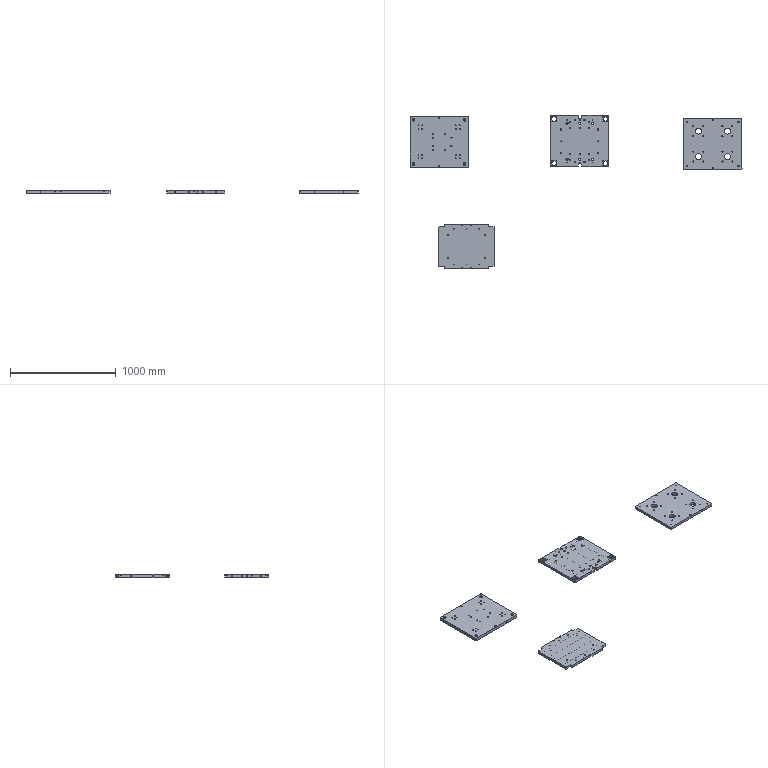NC program | Mastercam | posted with a generic post | part box 3140 x 1452 x 30 mm
Lines 6154 to 6493 of 6493:
N2080 T7 M6
N2090 G0 G90 G17 G54 X-248.05 Y-208.6 A0. S6000 M3
N2100 G43 H7 Z50. M8
N2110 Z1.2
N2120 G1 Z-1.25 F600.
N2130 X-248.45 F1000.
N2140 G3 X-248.85 Y-209. I0. J-.4
N2150 X-242. Y-215.85 I6.85 J0.
N2160 X-235.15 Y-209. I0. J6.85
N2170 X-242. Y-202.15 I-6.85 J0.
N2180 X-248.85 Y-209. I0. J-6.85
N2190 X-248.832 Y-209.5 I6.85 J0.
N2200 X-248.433 Y-209.87 I.399 J.03
N2210 X-248.404 Y-209.869 I0. J.4
N2220 G1 X-248.005 Y-209.84
N2230 G0 Z50.
N2240 X-245.55 Y-208.6
N2250 Z-9.8
N2260 G1 Z-12.25 F600.
N2270 X-245.95 F1000.
N2280 G3 X-246.35 Y-209. I0. J-.4
N2290 X-242. Y-213.35 I4.35 J0.
N2300 X-237.65 Y-209. I0. J4.35
N2310 X-242. Y-204.65 I-4.35 J0.
N2320 X-246.35 Y-209. I0. J-4.35
N2330 X-246.321 Y-209.499 I4.35 J0.
N2340 X-245.924 Y-209.853 I.397 J.046
N2350 X-245.878 Y-209.85 I0. J.4
N2360 G1 X-245.481 Y-209.805
N2370 G0 Z50.
N2380 X-6.05 Y-227.1
N2390 Z1.2
N2400 G1 Z-1.25 F600.
N2410 X-6.45 F1000.
N2420 G3 X-6.85 Y-227.5 I0. J-.4
N2430 X0. Y-234.35 I6.85 J0.
N2440 X6.85 Y-227.5 I0. J6.85
N2450 X0. Y-220.65 I-6.85 J0.
N2460 X-6.85 Y-227.5 I0. J-6.85
N2470 X-6.832 Y-228. I6.85 J0.
N2480 X-6.433 Y-228.37 I.399 J.03
N2490 X-6.404 Y-228.369 I0. J.4
N2500 G1 X-6.005 Y-228.34
N2510 G0 Z50.
N2520 X-3.55 Y-227.1
N2530 Z-9.8
N2540 G1 Z-12.25 F600.
N2550 X-3.95 F1000.
N2560 G3 X-4.35 Y-227.5 I0. J-.4
N2570 X0. Y-231.85 I4.35 J0.
N2580 X4.35 Y-227.5 I0. J4.35
N2590 X0. Y-223.15 I-4.35 J0.
N2600 X-4.35 Y-227.5 I0. J-4.35
N2610 X-4.321 Y-227.999 I4.35 J0.
N2620 X-3.924 Y-228.353 I.397 J.046
N2630 X-3.878 Y-228.35 I0. J.4
N2640 G1 X-3.481 Y-228.305
N2650 G0 Z50.
N2660 X235.95 Y-208.6
N2670 Z1.2
N2680 G1 Z-1.25 F600.
N2690 X235.55 F1000.
N2700 G3 X235.15 Y-209. I0. J-.4
N2710 X242. Y-215.85 I6.85 J0.
N2720 X248.85 Y-209. I0. J6.85
N2730 X242. Y-202.15 I-6.85 J0.
N2740 X235.15 Y-209. I0. J-6.85
N2750 X235.168 Y-209.5 I6.85 J0.
N2760 X235.567 Y-209.87 I.399 J.03
N2770 X235.596 Y-209.869 I0. J.4
N2780 G1 X235.995 Y-209.84
N2790 G0 Z50.
N2800 X238.45 Y-208.6
N2810 Z-9.8
N2820 G1 Z-12.25 F600.
N2830 X238.05 F1000.
N2840 G3 X237.65 Y-209. I0. J-.4
N2850 X242. Y-213.35 I4.35 J0.
N2860 X246.35 Y-209. I0. J4.35
N2870 X242. Y-204.65 I-4.35 J0.
N2880 X237.65 Y-209. I0. J-4.35
N2890 X237.679 Y-209.499 I4.35 J0.
N2900 X238.076 Y-209.853 I.397 J.046
N2910 X238.122 Y-209.85 I0. J.4
N2920 G1 X238.519 Y-209.805
N2930 G0 Z50.
N2940 X235.95 Y209.4
N2950 Z1.2
N2960 G1 Z-1.25 F600.
N2970 X235.55 F1000.
N2980 G3 X235.15 Y209. I0. J-.4
N2990 X242. Y202.15 I6.85 J0.
N3000 X248.85 Y209. I0. J6.85
N3010 X242. Y215.85 I-6.85 J0.
N3020 X235.15 Y209. I0. J-6.85
N3030 X235.168 Y208.5 I6.85 J0.
N3040 X235.567 Y208.13 I.399 J.03
N3050 X235.596 Y208.131 I0. J.4
N3060 G1 X235.995 Y208.16
N3070 G0 Z50.
N3080 X238.45 Y209.4
N3090 Z-9.8
N3100 G1 Z-12.25 F600.
N3110 X238.05 F1000.
N3120 G3 X237.65 Y209. I0. J-.4
N3130 X242. Y204.65 I4.35 J0.
N3140 X246.35 Y209. I0. J4.35
N3150 X242. Y213.35 I-4.35 J0.
N3160 X237.65 Y209. I0. J-4.35
N3170 X237.679 Y208.501 I4.35 J0.
N3180 X238.076 Y208.147 I.397 J.046
N3190 X238.122 Y208.15 I0. J.4
N3200 G1 X238.519 Y208.195
N3210 G0 Z50.
N3220 X-6.05 Y227.9
N3230 Z1.2
N3240 G1 Z-1.25 F600.
N3250 X-6.45 F1000.
N3260 G3 X-6.85 Y227.5 I0. J-.4
N3270 X0. Y220.65 I6.85 J0.
N3280 X6.85 Y227.5 I0. J6.85
N3290 X0. Y234.35 I-6.85 J0.
N3300 X-6.85 Y227.5 I0. J-6.85
N3310 X-6.832 Y227. I6.85 J0.
N3320 X-6.433 Y226.63 I.399 J.03
N3330 X-6.404 Y226.631 I0. J.4
N3340 G1 X-6.005 Y226.66
N3350 G0 Z50.
N3360 X-3.55 Y227.9
N3370 Z-9.8
N3380 G1 Z-12.25 F600.
N3390 X-3.95 F1000.
N3400 G3 X-4.35 Y227.5 I0. J-.4
N3410 X0. Y223.15 I4.35 J0.
N3420 X4.35 Y227.5 I0. J4.35
N3430 X0. Y231.85 I-4.35 J0.
N3440 X-4.35 Y227.5 I0. J-4.35
N3450 X-4.321 Y227.001 I4.35 J0.
N3460 X-3.924 Y226.647 I.397 J.046
N3470 X-3.878 Y226.65 I0. J.4
N3480 G1 X-3.481 Y226.695
N3490 G0 Z50.
N3500 X-248.05 Y209.4
N3510 Z1.2
N3520 G1 Z-1.25 F600.
N3530 X-248.45 F1000.
N3540 G3 X-248.85 Y209. I0. J-.4
N3550 X-242. Y202.15 I6.85 J0.
N3560 X-235.15 Y209. I0. J6.85
N3570 X-242. Y215.85 I-6.85 J0.
N3580 X-248.85 Y209. I0. J-6.85
N3590 X-248.832 Y208.5 I6.85 J0.
N3600 X-248.433 Y208.13 I.399 J.03
N3610 X-248.404 Y208.131 I0. J.4
N3620 G1 X-248.005 Y208.16
N3630 G0 Z50.
N3640 X-245.55 Y209.4
N3650 Z-9.8
N3660 G1 Z-12.25 F600.
N3670 X-245.95 F1000.
N3680 G3 X-246.35 Y209. I0. J-.4
N3690 X-242. Y204.65 I4.35 J0.
N3700 X-237.65 Y209. I0. J4.35
N3710 X-242. Y213.35 I-4.35 J0.
N3720 X-246.35 Y209. I0. J-4.35
N3730 X-246.321 Y208.501 I4.35 J0.
N3740 X-245.924 Y208.147 I.397 J.046
N3750 X-245.878 Y208.15 I0. J.4
N3760 G1 X-245.481 Y208.195
N3770 G0 Z50.
N3780 X-137.5 Y0.
N3790 G98 G81 Z-.7 R1. F200.
N3800 X137.5
N3810 G80
N3820 M5
N3830 G91 G0 G28 Z0. M9
N3840 A0.
N3850 M01
N3860 T15 M6
N3870 G0 G90 G17 G54 X-137.5 Y0. A0. S1200 M3
N3880 G43 H15 Z50. M8
N3890 G98 G83 Z-23. R1. Q2. F100.
N3900 X137.5
N3910 G80
N3920 M5
N3930 G91 G0 G28 Z0. M9
N3940 A0.
N3950 M01
N3960 T7 M6
N3970 G0 G90 G17 G54 X-138.15 Y.4 A0. S6000 M3
N3980 G43 H7 Z50. M8
N3990 Z1.2
N4000 G1 Z-1.5 F600.
N4010 X-138.55 F1000.
N4020 G3 X-138.95 Y0. I0. J-.4
N4030 X-137.5 Y-1.45 I1.45 J0.
N4040 X-136.05 Y0. I0. J1.45
N4050 X-137.5 Y1.45 I-1.45 J0.
N4060 X-138.95 Y0. I0. J-1.45
N4070 X-138.865 Y-.49 I1.45 J0.
N4080 X-138.488 Y-.755 I.377 J.135
N4090 X-138.353 Y-.731 I0. J.4
N4100 G1 X-137.977 Y-.596
N4110 G0 Z50.
N4120 X136.85 Y.4
N4130 Z1.2
N4140 G1 Z-1.5 F600.
N4150 X136.45 F1000.
N4160 G3 X136.05 Y0. I0. J-.4
N4170 X137.5 Y-1.45 I1.45 J0.
N4180 X138.95 Y0. I0. J1.45
N4190 X137.5 Y1.45 I-1.45 J0.
N4200 X136.05 Y0. I0. J-1.45
N4210 X136.135 Y-.49 I1.45 J0.
N4220 X136.512 Y-.755 I.377 J.135
N4230 X136.647 Y-.731 I0. J.4
N4240 G1 X137.023 Y-.596
N4250 G0 Z50.
G91G28X0.Y0.
N4260 S6250 M3
N4270 M9
N4280 X-227.5 Y0. Z10.
N4290 G98 G81 Z-.7 R1. F750.
N4300 X-198.5 Y10.
N4310 X-105. Y0.
N4320 X105.
N4330 X198.5 Y10.
N4340 X227.5 Y0.
N4350 G80
N4360 M5
N4370 G91 G0 G28 Z0.
N4380 A0.
N4390 M01
G91G28X0.Y0.
N4400 T15 M6
N4410 G0 G90 G17 G54 X-227.5 Y0. A0. S1200 M3
N4420 G43 H15 Z10. M8
N4430 G98 G83 Z-21. R1. Q2. F100.
N4440 X-198.5 Y10.
N4450 X-105. Y0.
N4460 X105.
N4470 X198.5 Y10.
N4480 X227.5 Y0.
N4490 G80
N4500 M5
N4510 G91 G0 G28 Z0. M9
N4520 A0.
N4530 M01
G91G28X0.Y0.
N4540 T7 M6
N4550 G0 G90 G17 G54 X-226.85 Y-.4 A0. S6000 M3
N4560 G43 H7 Z10.
N4570 Z1.2
N4580 G1 Z-1.5 F600.
N4590 X-226.45 F1000.
N4600 G3 X-226.05 Y0. I0. J.4
N4610 X-227.5 Y1.45 I-1.45 J0.
N4620 X-228.95 Y0. I0. J-1.45
N4630 X-227.5 Y-1.45 I1.45 J0.
N4640 X-226.05 Y0. I0. J1.45
N4650 X-226.135 Y.49 I-1.45 J0.
N4660 X-226.512 Y.755 I-.377 J-.135
N4670 X-226.647 Y.731 I0. J-.4
N4680 G1 X-227.023 Y.596
N4690 G0 Z10.
N4700 X199.15 Y9.6
N4710 Z1.2
N4720 G1 Z-1.5 F600.
N4730 X199.55 F1000.
N4740 G3 X199.95 Y10. I0. J.4
N4750 X198.5 Y11.45 I-1.45 J0.
N4760 X197.05 Y10. I0. J-1.45
N4770 X198.5 Y8.55 I1.45 J0.
N4780 X199.95 Y10. I0. J1.45
N4790 X199.865 Y10.49 I-1.45 J0.
N4800 X199.488 Y10.755 I-.377 J-.135
N4810 X199.353 Y10.731 I0. J-.4
N4820 G1 X198.977 Y10.596
N4830 G0 Z10.
N4840 X228.15 Y-.4
N4850 Z1.2
N4860 G1 Z-1.5 F600.
N4870 X228.55 F1000.
N4880 G3 X228.95 Y0. I0. J.4
N4890 X227.5 Y1.45 I-1.45 J0.
N4900 X226.05 Y0. I0. J-1.45
N4910 X227.5 Y-1.45 I1.45 J0.
N4920 X228.95 Y0. I0. J1.45
N4930 X228.865 Y.49 I-1.45 J0.
N4940 X228.488 Y.755 I-.377 J-.135
N4950 X228.353 Y.731 I0. J-.4
N4960 G1 X227.977 Y.596
N4970 G0 Z10.
N4980 X105.65 Y-.4
N4990 Z1.2
N5000 G1 Z-1.5 F600.
N5010 X106.05 F1000.
N5020 G3 X106.45 Y0. I0. J.4
N5030 X105. Y1.45 I-1.45 J0.
N5040 X103.55 Y0. I0. J-1.45
N5050 X105. Y-1.45 I1.45 J0.
N5060 X106.45 Y0. I0. J1.45
N5070 X106.365 Y.49 I-1.45 J0.
N5080 X105.988 Y.755 I-.377 J-.135
N5090 X105.853 Y.731 I0. J-.4
N5100 G1 X105.477 Y.596
N5110 G0 Z10.
N5120 X-104.35 Y-.4
N5130 Z1.2
N5140 G1 Z-1.5 F600.
N5150 X-103.95 F1000.
N5160 G3 X-103.55 Y0. I0. J.4
N5170 X-105. Y1.45 I-1.45 J0.
N5180 X-106.45 Y0. I0. J-1.45
N5190 X-105. Y-1.45 I1.45 J0.
N5200 X-103.55 Y0. I0. J1.45
N5210 X-103.635 Y.49 I-1.45 J0.
N5220 X-104.012 Y.755 I-.377 J-.135
N5230 X-104.147 Y.731 I0. J-.4
N5240 G1 X-104.523 Y.596
N5250 G0 Z10.
N5260 X-197.85 Y9.6
N5270 Z1.2
N5280 G1 Z-1.5 F600.
N5290 X-197.45 F1000.
N5300 G3 X-197.05 Y10. I0. J.4
N5310 X-198.5 Y11.45 I-1.45 J0.
N5320 X-199.95 Y10. I0. J-1.45
N5330 X-198.5 Y8.55 I1.45 J0.
N5340 X-197.05 Y10. I0. J1.45
N5350 X-197.135 Y10.49 I-1.45 J0.
N5360 X-197.512 Y10.755 I-.377 J-.135
N5370 X-197.647 Y10.731 I0. J-.4
N5380 G1 X-198.023 Y10.596
N5390 G0 Z10.
N5400 M5
N5410 G91 G28 Z0.
N5420 G28 X0. Y0. A0.
N5430 M30
%